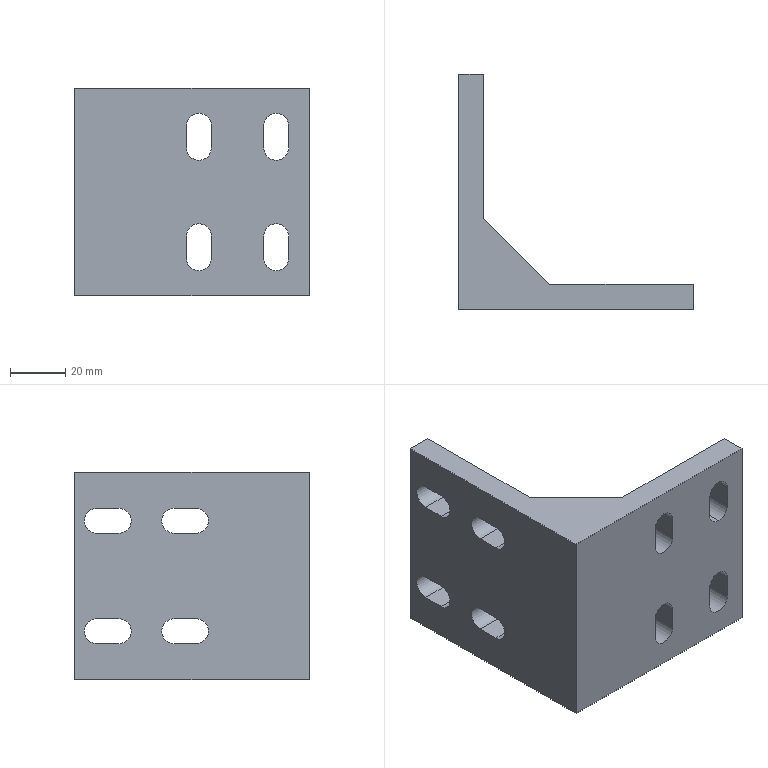Part | 1 solid | 49 faces | box 85 x 85 x 75 mm | volume 120511 mm3 | plane 25 | cylinder 24 | commonest cylinder face diameters 9 x24